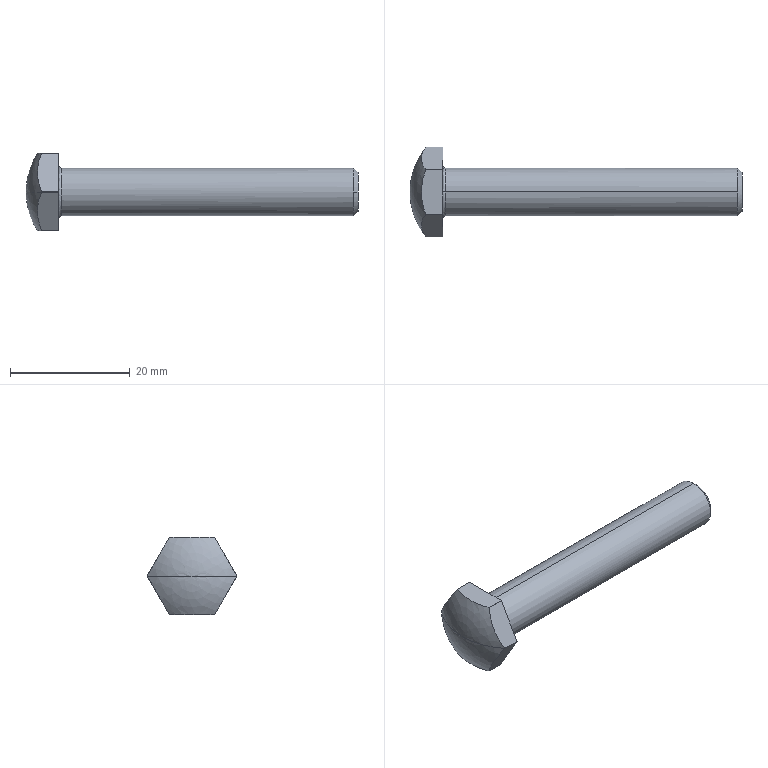Part | STEP file | 1_12 | 1 solid | 22 faces | volume 3160 mm3 | cylinder 8 | plane 8 | spline 4 | cone 2 | commonest cylinder face diameters 15 x6 8 x2